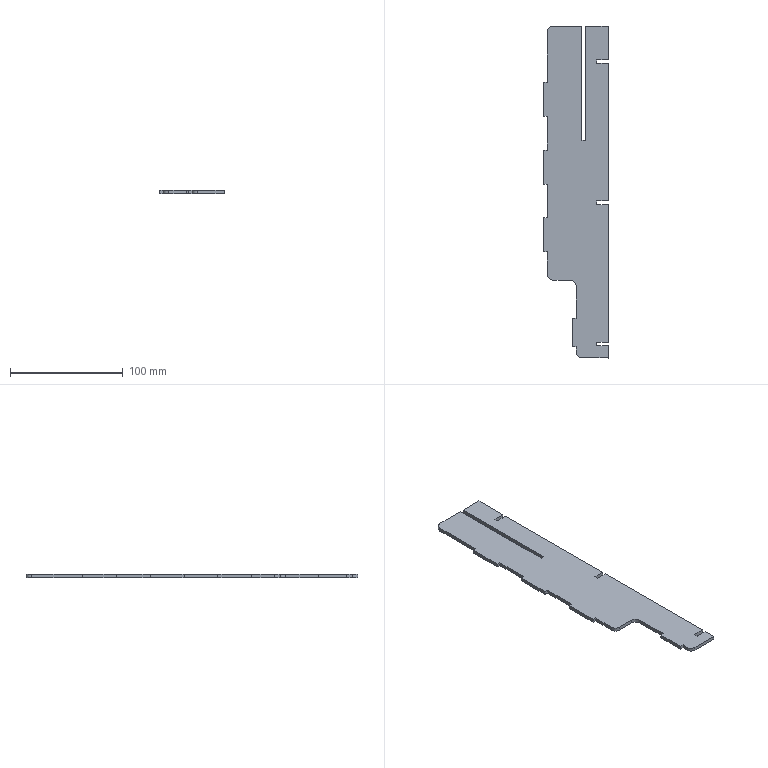Part | SolidWorks | features FlatPattern 1, SMBaseFlange 1, SheetMetal 1 | 1 solid | 44 faces | box 57 x 294.081 x 3.2 mm | volume 44908 mm3 | plane 40 | cylinder 4 | commonest cylinder face diameters 10 x4
STEP:
#1=CARTESIAN_POINT('',(-401.9,-209.357,0.));
#2=VERTEX_POINT('',#1);
#3=CARTESIAN_POINT('',(-378.4,-209.357,0.));
#4=VERTEX_POINT('',#3);
#5=CARTESIAN_POINT('',(-401.9,-209.357,0.));
#6=DIRECTION('',(1.,-0.00000003,0.));
#7=VECTOR('',#6,1000.);
#8=LINE('',#5,#7);
#9=EDGE_CURVE('',#2,#4,#8,.T.);
#10=ORIENTED_EDGE('',*,*,#9,.F.);
#11=CARTESIAN_POINT('',(-401.9,-209.357,-3.2));
#12=VERTEX_POINT('',#11);
#13=CARTESIAN_POINT('',(-401.9,-209.357,-3.2));
#14=DIRECTION('',(0.,0.,1.));
#15=VECTOR('',#14,1000.);
#16=LINE('',#13,#15);
#17=EDGE_CURVE('',#12,#2,#16,.T.);
#18=ORIENTED_EDGE('',*,*,#17,.F.);
#19=CARTESIAN_POINT('',(-378.4,-209.357,-3.2));
#20=VERTEX_POINT('',#19);
#21=CARTESIAN_POINT('',(-401.9,-209.357,-3.2));
#22=DIRECTION('',(1.,-0.00000003,0.));
#23=VECTOR('',#22,1000.);
#24=LINE('',#21,#23);
#25=EDGE_CURVE('',#12,#20,#24,.T.);
#26=ORIENTED_EDGE('',*,*,#25,.T.);
#27=CARTESIAN_POINT('',(-378.4,-209.357,-3.2));
#28=DIRECTION('',(0.,0.,1.));
#29=VECTOR('',#28,1000.);
#30=LINE('',#27,#29);
#31=EDGE_CURVE('',#20,#4,#30,.T.);
#32=ORIENTED_EDGE('',*,*,#31,.T.);
#33=EDGE_LOOP('',(#10,#18,#26,#32));
#34=FACE_OUTER_BOUND('',#33,.T.);
#35=CARTESIAN_POINT('',(-401.9,-209.357,-3.2));
#36=DIRECTION('',(-0.00000003,-1.,0.));
#37=DIRECTION('',(1.,-0.00000003,0.));
#38=AXIS2_PLACEMENT_3D('',#35,#36,#37);
#39=PLANE('',#38);
#40=ADVANCED_FACE('',(#34),#39,.T.);
#41=CARTESIAN_POINT('',(-406.9,-204.357,0.));
#42=VERTEX_POINT('',#41);
#43=CARTESIAN_POINT('',(-401.9,-204.357,0.));
#44=DIRECTION('',(0.,0.,1.));
#45=DIRECTION('',(-1.,0.,0.));
#46=AXIS2_PLACEMENT_3D('',#43,#44,#45);
#47=CIRCLE('',#46,5.);
#48=EDGE_CURVE('',#42,#2,#47,.T.);
#49=ORIENTED_EDGE('',*,*,#48,.F.);
#50=CARTESIAN_POINT('',(-406.9,-204.357,-3.2));
#51=VERTEX_POINT('',#50);
#52=CARTESIAN_POINT('',(-406.9,-204.357,-3.2));
#53=DIRECTION('',(0.,0.,1.));
#54=VECTOR('',#53,1000.);
#55=LINE('',#52,#54);
#56=EDGE_CURVE('',#51,#42,#55,.T.);
#57=ORIENTED_EDGE('',*,*,#56,.F.);
#58=CARTESIAN_POINT('',(-401.9,-204.357,-3.2));
#59=DIRECTION('',(0.,0.,1.));
#60=DIRECTION('',(-1.,0.,0.));
#61=AXIS2_PLACEMENT_3D('',#58,#59,#60);
#62=CIRCLE('',#61,5.);
#63=EDGE_CURVE('',#51,#12,#62,.T.);
#64=ORIENTED_EDGE('',*,*,#63,.T.);
#65=ORIENTED_EDGE('',*,*,#17,.T.);
#66=EDGE_LOOP('',(#49,#57,#64,#65));
#67=FACE_OUTER_BOUND('',#66,.T.);
#68=CARTESIAN_POINT('',(-401.9,-204.357,-3.2));
#69=DIRECTION('',(0.,0.,1.));
#70=DIRECTION('',(1.,0.,0.));
#71=AXIS2_PLACEMENT_3D('',#68,#69,#70);
#72=CYLINDRICAL_SURFACE('',#71,5.);
#73=ADVANCED_FACE('',(#67),#72,.T.);
#74=CARTESIAN_POINT('',(-406.9,-199.357,0.));
#75=VERTEX_POINT('',#74);
#76=CARTESIAN_POINT('',(-406.9,-199.357,0.));
#77=DIRECTION('',(0.,-1.,0.));
#78=VECTOR('',#77,1000.);
#79=LINE('',#76,#78);
#80=EDGE_CURVE('',#75,#42,#79,.T.);
#81=ORIENTED_EDGE('',*,*,#80,.F.);
#82=CARTESIAN_POINT('',(-406.9,-199.357,-3.2));
#83=VERTEX_POINT('',#82);
#84=CARTESIAN_POINT('',(-406.9,-199.357,-3.2));
#85=DIRECTION('',(0.,0.,1.));
#86=VECTOR('',#85,1000.);
#87=LINE('',#84,#86);
#88=EDGE_CURVE('',#83,#75,#87,.T.);
#89=ORIENTED_EDGE('',*,*,#88,.F.);
#90=CARTESIAN_POINT('',(-406.9,-199.357,-3.2));
#91=DIRECTION('',(0.,-1.,0.));
#92=VECTOR('',#91,1000.);
#93=LINE('',#90,#92);
#94=EDGE_CURVE('',#83,#51,#93,.T.);
#95=ORIENTED_EDGE('',*,*,#94,.T.);
#96=ORIENTED_EDGE('',*,*,#56,.T.);
#97=EDGE_LOOP('',(#81,#89,#95,#96));
#98=FACE_OUTER_BOUND('',#97,.T.);
#99=CARTESIAN_POINT('',(-406.9,-199.357,-3.2));
#100=DIRECTION('',(-1.,0.,0.));
#101=DIRECTION('',(0.,0.,1.));
#102=AXIS2_PLACEMENT_3D('',#99,#100,#101);
#103=PLANE('',#102);
#104=ADVANCED_FACE('',(#98),#103,.T.);
#105=CARTESIAN_POINT('',(-409.9,-199.357,0.));
#106=VERTEX_POINT('',#105);
#107=CARTESIAN_POINT('',(-409.9,-199.357,0.));
#108=DIRECTION('',(1.,0.,0.));
#109=VECTOR('',#108,1000.);
#110=LINE('',#107,#109);
#111=EDGE_CURVE('',#106,#75,#110,.T.);
#112=ORIENTED_EDGE('',*,*,#111,.F.);
#113=CARTESIAN_POINT('',(-409.9,-199.357,-3.2));
#114=VERTEX_POINT('',#113);
#115=CARTESIAN_POINT('',(-409.9,-199.357,-3.2));
#116=DIRECTION('',(0.,0.,1.));
#117=VECTOR('',#116,1000.);
#118=LINE('',#115,#117);
#119=EDGE_CURVE('',#114,#106,#118,.T.);
#120=ORIENTED_EDGE('',*,*,#119,.F.);
#121=CARTESIAN_POINT('',(-409.9,-199.357,-3.2));
#122=DIRECTION('',(1.,0.,0.));
#123=VECTOR('',#122,1000.);
#124=LINE('',#121,#123);
#125=EDGE_CURVE('',#114,#83,#124,.T.);
#126=ORIENTED_EDGE('',*,*,#125,.T.);
#127=ORIENTED_EDGE('',*,*,#88,.T.);
#128=EDGE_LOOP('',(#112,#120,#126,#127));
#129=FACE_OUTER_BOUND('',#128,.T.);
#130=CARTESIAN_POINT('',(-409.9,-199.357,-3.2));
#131=DIRECTION('',(0.,-1.,0.));
#132=DIRECTION('',(1.,0.,0.));
#133=AXIS2_PLACEMENT_3D('',#130,#131,#132);
#134=PLANE('',#133);
#135=ADVANCED_FACE('',(#129),#134,.T.);
#136=CARTESIAN_POINT('',(-409.9,-174.357,0.));
#137=VERTEX_POINT('',#136);
#138=CARTESIAN_POINT('',(-409.9,-174.357,0.));
#139=DIRECTION('',(0.,-1.,0.));
#140=VECTOR('',#139,1000.);
#141=LINE('',#138,#140);
#142=EDGE_CURVE('',#137,#106,#141,.T.);
#143=ORIENTED_EDGE('',*,*,#142,.F.);
#144=CARTESIAN_POINT('',(-409.9,-174.357,-3.2));
#145=VERTEX_POINT('',#144);
#146=CARTESIAN_POINT('',(-409.9,-174.357,-3.2));
#147=DIRECTION('',(0.,0.,1.));
#148=VECTOR('',#147,1000.);
#149=LINE('',#146,#148);
#150=EDGE_CURVE('',#145,#137,#149,.T.);
#151=ORIENTED_EDGE('',*,*,#150,.F.);
#152=CARTESIAN_POINT('',(-409.9,-174.357,-3.2));
#153=DIRECTION('',(0.,-1.,0.));
#154=VECTOR('',#153,1000.);
#155=LINE('',#152,#154);
#156=EDGE_CURVE('',#145,#114,#155,.T.);
#157=ORIENTED_EDGE('',*,*,#156,.T.);
#158=ORIENTED_EDGE('',*,*,#119,.T.);
#159=EDGE_LOOP('',(#143,#151,#157,#158));
#160=FACE_OUTER_BOUND('',#159,.T.);
#161=CARTESIAN_POINT('',(-409.9,-174.357,-3.2));
#162=DIRECTION('',(-1.,0.,0.));
#163=DIRECTION('',(0.,-1.,0.));
#164=AXIS2_PLACEMENT_3D('',#161,#162,#163);
#165=PLANE('',#164);
#166=ADVANCED_FACE('',(#160),#165,.T.);
#167=CARTESIAN_POINT('',(-406.9,-174.357,0.));
#168=VERTEX_POINT('',#167);
#169=CARTESIAN_POINT('',(-406.9,-174.357,0.));
#170=DIRECTION('',(-1.,0.,0.));
#171=VECTOR('',#170,1000.);
#172=LINE('',#169,#171);
#173=EDGE_CURVE('',#168,#137,#172,.T.);
#174=ORIENTED_EDGE('',*,*,#173,.F.);
#175=CARTESIAN_POINT('',(-406.9,-174.357,-3.2));
#176=VERTEX_POINT('',#175);
#177=CARTESIAN_POINT('',(-406.9,-174.357,-3.2));
#178=DIRECTION('',(0.,0.,1.));
#179=VECTOR('',#178,1000.);
#180=LINE('',#177,#179);
#181=EDGE_CURVE('',#176,#168,#180,.T.);
#182=ORIENTED_EDGE('',*,*,#181,.F.);
#183=CARTESIAN_POINT('',(-406.9,-174.357,-3.2));
#184=DIRECTION('',(-1.,0.,0.));
#185=VECTOR('',#184,1000.);
#186=LINE('',#183,#185);
#187=EDGE_CURVE('',#176,#145,#186,.T.);
#188=ORIENTED_EDGE('',*,*,#187,.T.);
#189=ORIENTED_EDGE('',*,*,#150,.T.);
#190=EDGE_LOOP('',(#174,#182,#188,#189));
#191=FACE_OUTER_BOUND('',#190,.T.);
#192=CARTESIAN_POINT('',(-406.9,-174.357,-3.2));
#193=DIRECTION('',(0.,1.,0.));
#194=DIRECTION('',(0.,0.,1.));
#195=AXIS2_PLACEMENT_3D('',#192,#193,#194);
#196=PLANE('',#195);
#197=ADVANCED_FACE('',(#191),#196,.T.);
#198=CARTESIAN_POINT('',(-406.9,-145.276,0.));
#199=VERTEX_POINT('',#198);
#200=CARTESIAN_POINT('',(-406.9,-145.276,0.));
#201=DIRECTION('',(0.000000012,-1.,0.));
#202=VECTOR('',#201,1000.);
#203=LINE('',#200,#202);
#204=EDGE_CURVE('',#199,#168,#203,.T.);
#205=ORIENTED_EDGE('',*,*,#204,.F.);
#206=CARTESIAN_POINT('',(-406.9,-145.276,-3.2));
#207=VERTEX_POINT('',#206);
#208=CARTESIAN_POINT('',(-406.9,-145.276,-3.2));
#209=DIRECTION('',(0.,0.,1.));
#210=VECTOR('',#209,1000.);
#211=LINE('',#208,#210);
#212=EDGE_CURVE('',#207,#199,#211,.T.);
#213=ORIENTED_EDGE('',*,*,#212,.F.);
#214=CARTESIAN_POINT('',(-406.9,-145.276,-3.2));
#215=DIRECTION('',(0.000000012,-1.,0.));
#216=VECTOR('',#215,1000.);
#217=LINE('',#214,#216);
#218=EDGE_CURVE('',#207,#176,#217,.T.);
#219=ORIENTED_EDGE('',*,*,#218,.T.);
#220=ORIENTED_EDGE('',*,*,#181,.T.);
#221=EDGE_LOOP('',(#205,#213,#219,#220));
#222=FACE_OUTER_BOUND('',#221,.T.);
#223=CARTESIAN_POINT('',(-406.9,-145.276,-3.2));
#224=DIRECTION('',(-1.,-0.000000012,0.));
#225=DIRECTION('',(0.000000012,-1.,0.));
#226=AXIS2_PLACEMENT_3D('',#223,#224,#225);
#227=PLANE('',#226);
#228=ADVANCED_FACE('',(#222),#227,.T.);
#229=CARTESIAN_POINT('',(-411.9,-140.276,0.));
#230=VERTEX_POINT('',#229);
#231=CARTESIAN_POINT('',(-411.9,-145.276,0.));
#232=DIRECTION('',(0.,0.,-1.));
#233=DIRECTION('',(-1.,0.,0.));
#234=AXIS2_PLACEMENT_3D('',#231,#232,#233);
#235=CIRCLE('',#234,5.);
#236=EDGE_CURVE('',#230,#199,#235,.T.);
#237=ORIENTED_EDGE('',*,*,#236,.F.);
#238=CARTESIAN_POINT('',(-411.9,-140.276,-3.2));
#239=VERTEX_POINT('',#238);
#240=CARTESIAN_POINT('',(-411.9,-140.276,-3.2));
#241=DIRECTION('',(0.,0.,1.));
#242=VECTOR('',#241,1000.);
#243=LINE('',#240,#242);
#244=EDGE_CURVE('',#239,#230,#243,.T.);
#245=ORIENTED_EDGE('',*,*,#244,.F.);
#246=CARTESIAN_POINT('',(-411.9,-145.276,-3.2));
#247=DIRECTION('',(0.,0.,-1.));
#248=DIRECTION('',(-1.,0.,0.));
#249=AXIS2_PLACEMENT_3D('',#246,#247,#248);
#250=CIRCLE('',#249,5.);
#251=EDGE_CURVE('',#239,#207,#250,.T.);
#252=ORIENTED_EDGE('',*,*,#251,.T.);
#253=ORIENTED_EDGE('',*,*,#212,.T.);
#254=EDGE_LOOP('',(#237,#245,#252,#253));
#255=FACE_OUTER_BOUND('',#254,.T.);
#256=CARTESIAN_POINT('',(-411.9,-145.276,-3.2));
#257=DIRECTION('',(0.,0.,1.));
#258=DIRECTION('',(1.,0.,0.));
#259=AXIS2_PLACEMENT_3D('',#256,#257,#258);
#260=CYLINDRICAL_SURFACE('',#259,5.);
#261=ADVANCED_FACE('',(#255),#260,.F.);
#262=CARTESIAN_POINT('',(-427.4,-140.276,0.));
#263=VERTEX_POINT('',#262);
#264=CARTESIAN_POINT('',(-427.4,-140.276,0.));
#265=DIRECTION('',(1.,0.,0.));
#266=VECTOR('',#265,1000.);
#267=LINE('',#264,#266);
#268=EDGE_CURVE('',#263,#230,#267,.T.);
#269=ORIENTED_EDGE('',*,*,#268,.F.);
#270=CARTESIAN_POINT('',(-427.4,-140.276,-3.2));
#271=VERTEX_POINT('',#270);
#272=CARTESIAN_POINT('',(-427.4,-140.276,-3.2));
#273=DIRECTION('',(0.,0.,1.));
#274=VECTOR('',#273,1000.);
#275=LINE('',#272,#274);
#276=EDGE_CURVE('',#271,#263,#275,.T.);
#277=ORIENTED_EDGE('',*,*,#276,.F.);
#278=CARTESIAN_POINT('',(-427.4,-140.276,-3.2));
#279=DIRECTION('',(1.,0.,0.));
#280=VECTOR('',#279,1000.);
#281=LINE('',#278,#280);
#282=EDGE_CURVE('',#271,#239,#281,.T.);
#283=ORIENTED_EDGE('',*,*,#282,.T.);
#284=ORIENTED_EDGE('',*,*,#244,.T.);
#285=EDGE_LOOP('',(#269,#277,#283,#284));
#286=FACE_OUTER_BOUND('',#285,.T.);
#287=CARTESIAN_POINT('',(-427.4,-140.276,-3.2));
#288=DIRECTION('',(0.,-1.,0.));
#289=DIRECTION('',(0.,0.,-1.));
#290=AXIS2_PLACEMENT_3D('',#287,#288,#289);
#291=PLANE('',#290);
#292=ADVANCED_FACE('',(#286),#291,.T.);
#293=CARTESIAN_POINT('',(-432.4,-135.276,0.));
#294=VERTEX_POINT('',#293);
#295=CARTESIAN_POINT('',(-427.4,-135.276,0.));
#296=DIRECTION('',(0.,0.,1.));
#297=DIRECTION('',(-1.,0.,0.));
#298=AXIS2_PLACEMENT_3D('',#295,#296,#297);
#299=CIRCLE('',#298,5.);
#300=EDGE_CURVE('',#294,#263,#299,.T.);
#301=ORIENTED_EDGE('',*,*,#300,.F.);
#302=CARTESIAN_POINT('',(-432.4,-135.276,-3.2));
#303=VERTEX_POINT('',#302);
#304=CARTESIAN_POINT('',(-432.4,-135.276,-3.2));
#305=DIRECTION('',(0.,0.,1.));
#306=VECTOR('',#305,1000.);
#307=LINE('',#304,#306);
#308=EDGE_CURVE('',#303,#294,#307,.T.);
#309=ORIENTED_EDGE('',*,*,#308,.F.);
#310=CARTESIAN_POINT('',(-427.4,-135.276,-3.2));
#311=DIRECTION('',(0.,0.,1.));
#312=DIRECTION('',(-1.,0.,0.));
#313=AXIS2_PLACEMENT_3D('',#310,#311,#312);
#314=CIRCLE('',#313,5.);
#315=EDGE_CURVE('',#303,#271,#314,.T.);
#316=ORIENTED_EDGE('',*,*,#315,.T.);
#317=ORIENTED_EDGE('',*,*,#276,.T.);
#318=EDGE_LOOP('',(#301,#309,#316,#317));
#319=FACE_OUTER_BOUND('',#318,.T.);
#320=CARTESIAN_POINT('',(-427.4,-135.276,-3.2));
#321=DIRECTION('',(0.,0.,1.));
#322=DIRECTION('',(1.,0.,0.));
#323=AXIS2_PLACEMENT_3D('',#320,#321,#322);
#324=CYLINDRICAL_SURFACE('',#323,5.);
#325=ADVANCED_FACE('',(#319),#324,.T.);
#326=CARTESIAN_POINT('',(-432.4,-115.276,0.));
#327=VERTEX_POINT('',#326);
#328=CARTESIAN_POINT('',(-432.4,-135.276,0.));
#329=DIRECTION('',(0.,-1.,0.));
#330=VECTOR('',#329,1000.);
#331=LINE('',#328,#330);
#332=EDGE_CURVE('',#327,#294,#331,.T.);
#333=ORIENTED_EDGE('',*,*,#332,.F.);
#334=CARTESIAN_POINT('',(-432.4,-115.276,-3.2));
#335=VERTEX_POINT('',#334);
#336=CARTESIAN_POINT('',(-432.4,-115.276,-3.2));
#337=DIRECTION('',(0.,0.,1.));
#338=VECTOR('',#337,1000.);
#339=LINE('',#336,#338);
#340=EDGE_CURVE('',#335,#327,#339,.T.);
#341=ORIENTED_EDGE('',*,*,#340,.F.);
#342=CARTESIAN_POINT('',(-432.4,-135.276,-3.2));
#343=DIRECTION('',(0.,-1.,0.));
#344=VECTOR('',#343,1000.);
#345=LINE('',#342,#344);
#346=EDGE_CURVE('',#335,#303,#345,.T.);
#347=ORIENTED_EDGE('',*,*,#346,.T.);
#348=ORIENTED_EDGE('',*,*,#308,.T.);
#349=EDGE_LOOP('',(#333,#341,#347,#348));
#350=FACE_OUTER_BOUND('',#349,.T.);
#351=CARTESIAN_POINT('',(-432.4,-135.276,-3.2));
#352=DIRECTION('',(-1.,0.,0.));
#353=DIRECTION('',(0.,0.,1.));
#354=AXIS2_PLACEMENT_3D('',#351,#352,#353);
#355=PLANE('',#354);
#356=ADVANCED_FACE('',(#350),#355,.T.);
#357=CARTESIAN_POINT('',(-435.4,-115.276,0.));
#358=VERTEX_POINT('',#357);
#359=CARTESIAN_POINT('',(-435.4,-115.276,0.));
#360=DIRECTION('',(1.,0.,0.));
#361=VECTOR('',#360,1000.);
#362=LINE('',#359,#361);
#363=EDGE_CURVE('',#358,#327,#362,.T.);
#364=ORIENTED_EDGE('',*,*,#363,.F.);
#365=CARTESIAN_POINT('',(-435.4,-115.276,-3.2));
#366=VERTEX_POINT('',#365);
#367=CARTESIAN_POINT('',(-435.4,-115.276,-3.2));
#368=DIRECTION('',(0.,0.,1.));
#369=VECTOR('',#368,1000.);
#370=LINE('',#367,#369);
#371=EDGE_CURVE('',#366,#358,#370,.T.);
#372=ORIENTED_EDGE('',*,*,#371,.F.);
#373=CARTESIAN_POINT('',(-435.4,-115.276,-3.2));
#374=DIRECTION('',(1.,0.,0.));
#375=VECTOR('',#374,1000.);
#376=LINE('',#373,#375);
#377=EDGE_CURVE('',#366,#335,#376,.T.);
#378=ORIENTED_EDGE('',*,*,#377,.T.);
#379=ORIENTED_EDGE('',*,*,#340,.T.);
#380=EDGE_LOOP('',(#364,#372,#378,#379));
#381=FACE_OUTER_BOUND('',#380,.T.);
#382=CARTESIAN_POINT('',(-435.4,-115.276,-3.2));
#383=DIRECTION('',(0.,-1.,0.));
#384=DIRECTION('',(0.,0.,-1.));
#385=AXIS2_PLACEMENT_3D('',#382,#383,#384);
#386=PLANE('',#385);
#387=ADVANCED_FACE('',(#381),#386,.T.);
#388=CARTESIAN_POINT('',(-435.4,-85.276,0.));
#389=VERTEX_POINT('',#388);
#390=CARTESIAN_POINT('',(-435.4,-85.276,0.));
#391=DIRECTION('',(0.,-1.,0.));
#392=VECTOR('',#391,1000.);
#393=LINE('',#390,#392);
#394=EDGE_CURVE('',#389,#358,#393,.T.);
#395=ORIENTED_EDGE('',*,*,#394,.F.);
#396=CARTESIAN_POINT('',(-435.4,-85.276,-3.2));
#397=VERTEX_POINT('',#396);
#398=CARTESIAN_POINT('',(-435.4,-85.276,-3.2));
#399=DIRECTION('',(0.,0.,1.));
#400=VECTOR('',#399,1000.);
#401=LINE('',#398,#400);
#402=EDGE_CURVE('',#397,#389,#401,.T.);
#403=ORIENTED_EDGE('',*,*,#402,.F.);
#404=CARTESIAN_POINT('',(-435.4,-85.276,-3.2));
#405=DIRECTION('',(0.,-1.,0.));
#406=VECTOR('',#405,1000.);
#407=LINE('',#404,#406);
#408=EDGE_CURVE('',#397,#366,#407,.T.);
#409=ORIENTED_EDGE('',*,*,#408,.T.);
#410=ORIENTED_EDGE('',*,*,#371,.T.);
#411=EDGE_LOOP('',(#395,#403,#409,#410));
#412=FACE_OUTER_BOUND('',#411,.T.);
#413=CARTESIAN_POINT('',(-435.4,-85.276,-3.2));
#414=DIRECTION('',(-1.,0.,0.));
#415=DIRECTION('',(0.,0.,1.));
#416=AXIS2_PLACEMENT_3D('',#413,#414,#415);
#417=PLANE('',#416);
#418=ADVANCED_FACE('',(#412),#417,.T.);
#419=CARTESIAN_POINT('',(-432.4,-85.276,0.));
#420=VERTEX_POINT('',#419);
#421=CARTESIAN_POINT('',(-432.4,-85.276,0.));
#422=DIRECTION('',(-1.,0.,0.));
#423=VECTOR('',#422,1000.);
#424=LINE('',#421,#423);
#425=EDGE_CURVE('',#420,#389,#424,.T.);
#426=ORIENTED_EDGE('',*,*,#425,.F.);
#427=CARTESIAN_POINT('',(-432.4,-85.276,-3.2));
#428=VERTEX_POINT('',#427);
#429=CARTESIAN_POINT('',(-432.4,-85.276,-3.2));
#430=DIRECTION('',(0.,0.,1.));
#431=VECTOR('',#430,1000.);
#432=LINE('',#429,#431);
#433=EDGE_CURVE('',#428,#420,#432,.T.);
#434=ORIENTED_EDGE('',*,*,#433,.F.);
#435=CARTESIAN_POINT('',(-432.4,-85.276,-3.2));
#436=DIRECTION('',(-1.,0.,0.));
#437=VECTOR('',#436,1000.);
#438=LINE('',#435,#437);
#439=EDGE_CURVE('',#428,#397,#438,.T.);
#440=ORIENTED_EDGE('',*,*,#439,.T.);
#441=ORIENTED_EDGE('',*,*,#402,.T.);
#442=EDGE_LOOP('',(#426,#434,#440,#441));
#443=FACE_OUTER_BOUND('',#442,.T.);
#444=CARTESIAN_POINT('',(-432.4,-85.276,-3.2));
#445=DIRECTION('',(0.,1.,0.));
#446=DIRECTION('',(0.,0.,1.));
#447=AXIS2_PLACEMENT_3D('',#444,#445,#446);
#448=PLANE('',#447);
#449=ADVANCED_FACE('',(#443),#448,.T.);
#450=CARTESIAN_POINT('',(-432.4,-55.276,0.));
#451=VERTEX_POINT('',#450);
#452=CARTESIAN_POINT('',(-432.4,-85.276,0.));
#453=DIRECTION('',(0.,-1.,0.));
#454=VECTOR('',#453,1000.);
#455=LINE('',#452,#454);
#456=EDGE_CURVE('',#451,#420,#455,.T.);
#457=ORIENTED_EDGE('',*,*,#456,.F.);
#458=CARTESIAN_POINT('',(-432.4,-55.276,-3.2));
#459=VERTEX_POINT('',#458);
#460=CARTESIAN_POINT('',(-432.4,-55.276,-3.2));
#461=DIRECTION('',(0.,0.,1.));
#462=VECTOR('',#461,1000.);
#463=LINE('',#460,#462);
#464=EDGE_CURVE('',#459,#451,#463,.T.);
#465=ORIENTED_EDGE('',*,*,#464,.F.);
#466=CARTESIAN_POINT('',(-432.4,-85.276,-3.2));
#467=DIRECTION('',(0.,-1.,0.));
#468=VECTOR('',#467,1000.);
#469=LINE('',#466,#468);
#470=EDGE_CURVE('',#459,#428,#469,.T.);
#471=ORIENTED_EDGE('',*,*,#470,.T.);
#472=ORIENTED_EDGE('',*,*,#433,.T.);
#473=EDGE_LOOP('',(#457,#465,#471,#472));
#474=FACE_OUTER_BOUND('',#473,.T.);
#475=CARTESIAN_POINT('',(-432.4,-85.276,-3.2));
#476=DIRECTION('',(-1.,0.,0.));
#477=DIRECTION('',(0.,0.,1.));
#478=AXIS2_PLACEMENT_3D('',#475,#476,#477);
#479=PLANE('',#478);
#480=ADVANCED_FACE('',(#474),#479,.T.);
#481=CARTESIAN_POINT('',(-435.4,-55.276,0.));
#482=VERTEX_POINT('',#481);
#483=CARTESIAN_POINT('',(-435.4,-55.276,0.));
#484=DIRECTION('',(1.,0.,0.));
#485=VECTOR('',#484,1000.);
#486=LINE('',#483,#485);
#487=EDGE_CURVE('',#482,#451,#486,.T.);
#488=ORIENTED_EDGE('',*,*,#487,.F.);
#489=CARTESIAN_POINT('',(-435.4,-55.276,-3.2));
#490=VERTEX_POINT('',#489);
#491=CARTESIAN_POINT('',(-435.4,-55.276,-3.2));
#492=DIRECTION('',(0.,0.,1.));
#493=VECTOR('',#492,1000.);
#494=LINE('',#491,#493);
#495=EDGE_CURVE('',#490,#482,#494,.T.);
#496=ORIENTED_EDGE('',*,*,#495,.F.);
#497=CARTESIAN_POINT('',(-435.4,-55.276,-3.2));
#498=DIRECTION('',(1.,0.,0.));
#499=VECTOR('',#498,1000.);
#500=LINE('',#497,#499);
#501=EDGE_CURVE('',#490,#459,#500,.T.);
#502=ORIENTED_EDGE('',*,*,#501,.T.);
#503=ORIENTED_EDGE('',*,*,#464,.T.);
#504=EDGE_LOOP('',(#488,#496,#502,#503));
#505=FACE_OUTER_BOUND('',#504,.T.);
#506=CARTESIAN_POINT('',(-435.4,-55.276,-3.2));
#507=DIRECTION('',(0.,-1.,0.));
#508=DIRECTION('',(0.,0.,-1.));
#509=AXIS2_PLACEMENT_3D('',#506,#507,#508);
#510=PLANE('',#509);
#511=ADVANCED_FACE('',(#505),#510,.T.);
#512=CARTESIAN_POINT('',(-435.4,-25.276,0.));
#513=VERTEX_POINT('',#512);
#514=CARTESIAN_POINT('',(-435.4,-25.276,0.));
#515=DIRECTION('',(0.,-1.,0.));
#516=VECTOR('',#515,1000.);
#517=LINE('',#514,#516);
#518=EDGE_CURVE('',#513,#482,#517,.T.);
#519=ORIENTED_EDGE('',*,*,#518,.F.);
#520=CARTESIAN_POINT('',(-435.4,-25.276,-3.2));
#521=VERTEX_POINT('',#520);
#522=CARTESIAN_POINT('',(-435.4,-25.276,-3.2));
#523=DIRECTION('',(0.,0.,1.));
#524=VECTOR('',#523,1000.);
#525=LINE('',#522,#524);
#526=EDGE_CURVE('',#521,#513,#525,.T.);
#527=ORIENTED_EDGE('',*,*,#526,.F.);
#528=CARTESIAN_POINT('',(-435.4,-25.276,-3.2));
#529=DIRECTION('',(0.,-1.,0.));
#530=VECTOR('',#529,1000.);
#531=LINE('',#528,#530);
#532=EDGE_CURVE('',#521,#490,#531,.T.);
#533=ORIENTED_EDGE('',*,*,#532,.T.);
#534=ORIENTED_EDGE('',*,*,#495,.T.);
#535=EDGE_LOOP('',(#519,#527,#533,#534));
#536=FACE_OUTER_BOUND('',#535,.T.);
#537=CARTESIAN_POINT('',(-435.4,-25.276,-3.2));
#538=DIRECTION('',(-1.,0.,0.));
#539=DIRECTION('',(0.,0.,1.));
#540=AXIS2_PLACEMENT_3D('',#537,#538,#539);
#541=PLANE('',#540);
#542=ADVANCED_FACE('',(#536),#541,.T.);
#543=CARTESIAN_POINT('',(-432.4,-25.276,0.));
#544=VERTEX_POINT('',#543);
#545=CARTESIAN_POINT('',(-432.4,-25.276,0.));
#546=DIRECTION('',(-1.,0.,0.));
#547=VECTOR('',#546,1000.);
#548=LINE('',#545,#547);
#549=EDGE_CURVE('',#544,#513,#548,.T.);
#550=ORIENTED_EDGE('',*,*,#549,.F.);
#551=CARTESIAN_POINT('',(-432.4,-25.276,-3.2));
#552=VERTEX_POINT('',#551);
#553=CARTESIAN_POINT('',(-432.4,-25.276,-3.2));
#554=DIRECTION('',(0.,0.,1.));
#555=VECTOR('',#554,1000.);
#556=LINE('',#553,#555);
#557=EDGE_CURVE('',#552,#544,#556,.T.);
#558=ORIENTED_EDGE('',*,*,#557,.F.);
#559=CARTESIAN_POINT('',(-432.4,-25.276,-3.2));
#560=DIRECTION('',(-1.,0.,0.));
#561=VECTOR('',#560,1000.);
#562=LINE('',#559,#561);
#563=EDGE_CURVE('',#552,#521,#562,.T.);
#564=ORIENTED_EDGE('',*,*,#563,.T.);
#565=ORIENTED_EDGE('',*,*,#526,.T.);
#566=EDGE_LOOP('',(#550,#558,#564,#565));
#567=FACE_OUTER_BOUND('',#566,.T.);
#568=CARTESIAN_POINT('',(-432.4,-25.276,-3.2));
#569=DIRECTION('',(0.,1.,0.));
#570=DIRECTION('',(0.,0.,1.));
#571=AXIS2_PLACEMENT_3D('',#568,#569,#570);
#572=PLANE('',#571);
#573=ADVANCED_FACE('',(#567),#572,.T.);
#574=CARTESIAN_POINT('',(-432.4,4.724,0.));
#575=VERTEX_POINT('',#574);
#576=CARTESIAN_POINT('',(-432.4,-25.276,0.));
#577=DIRECTION('',(0.,-1.,0.));
#578=VECTOR('',#577,1000.);
#579=LINE('',#576,#578);
#580=EDGE_CURVE('',#575,#544,#579,.T.);
#581=ORIENTED_EDGE('',*,*,#580,.F.);
#582=CARTESIAN_POINT('',(-432.4,4.724,-3.2));
#583=VERTEX_POINT('',#582);
#584=CARTESIAN_POINT('',(-432.4,4.724,-3.2));
#585=DIRECTION('',(0.,0.,1.));
#586=VECTOR('',#585,1000.);
#587=LINE('',#584,#586);
#588=EDGE_CURVE('',#583,#575,#587,.T.);
#589=ORIENTED_EDGE('',*,*,#588,.F.);
#590=CARTESIAN_POINT('',(-432.4,-25.276,-3.2));
#591=DIRECTION('',(0.,-1.,0.));
#592=VECTOR('',#591,1000.);
#593=LINE('',#590,#592);
#594=EDGE_CURVE('',#583,#552,#593,.T.);
#595=ORIENTED_EDGE('',*,*,#594,.T.);
#596=ORIENTED_EDGE('',*,*,#557,.T.);
#597=EDGE_LOOP('',(#581,#589,#595,#596));
#598=FACE_OUTER_BOUND('',#597,.T.);
#599=CARTESIAN_POINT('',(-432.4,-25.276,-3.2));
#600=DIRECTION('',(-1.,0.,0.));
#601=DIRECTION('',(0.,0.,1.));
#602=AXIS2_PLACEMENT_3D('',#599,#600,#601);
#603=PLANE('',#602);
#604=ADVANCED_FACE('',(#598),#603,.T.);
#605=CARTESIAN_POINT('',(-435.4,4.724,0.));
#606=VERTEX_POINT('',#605);
#607=CARTESIAN_POINT('',(-435.4,4.724,0.));
#608=DIRECTION('',(1.,0.,0.));
#609=VECTOR('',#608,1000.);
#610=LINE('',#607,#609);
#611=EDGE_CURVE('',#606,#575,#610,.T.);
#612=ORIENTED_EDGE('',*,*,#611,.F.);
#613=CARTESIAN_POINT('',(-435.4,4.724,-3.2));
#614=VERTEX_POINT('',#613);
#615=CARTESIAN_POINT('',(-435.4,4.724,-3.2));
#616=DIRECTION('',(0.,0.,1.));
#617=VECTOR('',#616,1000.);
#618=LINE('',#615,#617);
#619=EDGE_CURVE('',#614,#606,#618,.T.);
#620=ORIENTED_EDGE('',*,*,#619,.F.);
#621=CARTESIAN_POINT('',(-435.4,4.724,-3.2));
#622=DIRECTION('',(1.,0.,0.));
#623=VECTOR('',#622,1000.);
#624=LINE('',#621,#623);
#625=EDGE_CURVE('',#614,#583,#624,.T.);
#626=ORIENTED_EDGE('',*,*,#625,.T.);
#627=ORIENTED_EDGE('',*,*,#588,.T.);
#628=EDGE_LOOP('',(#612,#620,#626,#627));
#629=FACE_OUTER_BOUND('',#628,.T.);
#630=CARTESIAN_POINT('',(-435.4,4.724,-3.2));
#631=DIRECTION('',(0.,-1.,0.));
#632=DIRECTION('',(0.,0.,-1.));
#633=AXIS2_PLACEMENT_3D('',#630,#631,#632);
#634=PLANE('',#633);
#635=ADVANCED_FACE('',(#629),#634,.T.);
#636=CARTESIAN_POINT('',(-435.4,34.724,0.));
#637=VERTEX_POINT('',#636);
#638=CARTESIAN_POINT('',(-435.4,34.724,0.));
#639=DIRECTION('',(0.,-1.,0.));
#640=VECTOR('',#639,1000.);
#641=LINE('',#638,#640);
#642=EDGE_CURVE('',#637,#606,#641,.T.);
#643=ORIENTED_EDGE('',*,*,#642,.F.);
#644=CARTESIAN_POINT('',(-435.4,34.724,-3.2));
#645=VERTEX_POINT('',#644);
#646=CARTESIAN_POINT('',(-435.4,34.724,-3.2));
#647=DIRECTION('',(0.,0.,1.));
#648=VECTOR('',#647,1000.);
#649=LINE('',#646,#648);
#650=EDGE_CURVE('',#645,#637,#649,.T.);
#651=ORIENTED_EDGE('',*,*,#650,.F.);
#652=CARTESIAN_POINT('',(-435.4,34.724,-3.2));
#653=DIRECTION('',(0.,-1.,0.));
#654=VECTOR('',#653,1000.);
#655=LINE('',#652,#654);
#656=EDGE_CURVE('',#645,#614,#655,.T.);
#657=ORIENTED_EDGE('',*,*,#656,.T.);
#658=ORIENTED_EDGE('',*,*,#619,.T.);
#659=EDGE_LOOP('',(#643,#651,#657,#658));
#660=FACE_OUTER_BOUND('',#659,.T.);
#661=CARTESIAN_POINT('',(-435.4,34.724,-3.2));
#662=DIRECTION('',(-1.,0.,0.));
#663=DIRECTION('',(0.,0.,1.));
#664=AXIS2_PLACEMENT_3D('',#661,#662,#663);
#665=PLANE('',#664);
#666=ADVANCED_FACE('',(#660),#665,.T.);
#667=CARTESIAN_POINT('',(-432.4,34.724,0.));
#668=VERTEX_POINT('',#667);
#669=CARTESIAN_POINT('',(-432.4,34.724,0.));
#670=DIRECTION('',(-1.,0.,0.));
#671=VECTOR('',#670,1000.);
#672=LINE('',#669,#671);
#673=EDGE_CURVE('',#668,#637,#672,.T.);
#674=ORIENTED_EDGE('',*,*,#673,.F.);
#675=CARTESIAN_POINT('',(-432.4,34.724,-3.2));
#676=VERTEX_POINT('',#675);
#677=CARTESIAN_POINT('',(-432.4,34.724,-3.2));
#678=DIRECTION('',(0.,0.,1.));
#679=VECTOR('',#678,1000.);
#680=LINE('',#677,#679);
#681=EDGE_CURVE('',#676,#668,#680,.T.);
#682=ORIENTED_EDGE('',*,*,#681,.F.);
#683=CARTESIAN_POINT('',(-432.4,34.724,-3.2));
#684=DIRECTION('',(-1.,0.,0.));
#685=VECTOR('',#684,1000.);
#686=LINE('',#683,#685);
#687=EDGE_CURVE('',#676,#645,#686,.T.);
#688=ORIENTED_EDGE('',*,*,#687,.T.);
#689=ORIENTED_EDGE('',*,*,#650,.T.);
#690=EDGE_LOOP('',(#674,#682,#688,#689));
#691=FACE_OUTER_BOUND('',#690,.T.);
#692=CARTESIAN_POINT('',(-432.4,34.724,-3.2));
#693=DIRECTION('',(0.,1.,0.));
#694=DIRECTION('',(0.,0.,1.));
#695=AXIS2_PLACEMENT_3D('',#692,#693,#694);
#696=PLANE('',#695);
#697=ADVANCED_FACE('',(#691),#696,.T.);
#698=CARTESIAN_POINT('',(-432.4,79.724,0.));
#699=VERTEX_POINT('',#698);
#700=CARTESIAN_POINT('',(-432.4,34.724,0.));
#701=DIRECTION('',(0.,-1.,0.));
#702=VECTOR('',#701,1000.);
#703=LINE('',#700,#702);
#704=EDGE_CURVE('',#699,#668,#703,.T.);
#705=ORIENTED_EDGE('',*,*,#704,.F.);
#706=CARTESIAN_POINT('',(-432.4,79.724,-3.2));
#707=VERTEX_POINT('',#706);
#708=CARTESIAN_POINT('',(-432.4,79.724,-3.2));
#709=DIRECTION('',(0.,0.,1.));
#710=VECTOR('',#709,1000.);
#711=LINE('',#708,#710);
#712=EDGE_CURVE('',#707,#699,#711,.T.);
#713=ORIENTED_EDGE('',*,*,#712,.F.);
#714=CARTESIAN_POINT('',(-432.4,34.724,-3.2));
#715=DIRECTION('',(0.,-1.,0.));
#716=VECTOR('',#715,1000.);
#717=LINE('',#714,#716);
#718=EDGE_CURVE('',#707,#676,#717,.T.);
#719=ORIENTED_EDGE('',*,*,#718,.T.);
#720=ORIENTED_EDGE('',*,*,#681,.T.);
#721=EDGE_LOOP('',(#705,#713,#719,#720));
#722=FACE_OUTER_BOUND('',#721,.T.);
#723=CARTESIAN_POINT('',(-432.4,34.724,-3.2));
#724=DIRECTION('',(-1.,0.,0.));
#725=DIRECTION('',(0.,0.,1.));
#726=AXIS2_PLACEMENT_3D('',#723,#724,#725);
#727=PLANE('',#726);
#728=ADVANCED_FACE('',(#722),#727,.T.);
#729=CARTESIAN_POINT('',(-427.4,84.724,0.));
#730=VERTEX_POINT('',#729);
#731=CARTESIAN_POINT('',(-427.4,79.724,0.));
#732=DIRECTION('',(0.,0.,1.));
#733=DIRECTION('',(1.,0.,0.));
#734=AXIS2_PLACEMENT_3D('',#731,#732,#733);
#735=CIRCLE('',#734,5.);
#736=EDGE_CURVE('',#730,#699,#735,.T.);
#737=ORIENTED_EDGE('',*,*,#736,.F.);
#738=CARTESIAN_POINT('',(-427.4,84.724,-3.2));
#739=VERTEX_POINT('',#738);
#740=CARTESIAN_POINT('',(-427.4,84.724,-3.2));
#741=DIRECTION('',(0.,0.,1.));
#742=VECTOR('',#741,1000.);
#743=LINE('',#740,#742);
#744=EDGE_CURVE('',#739,#730,#743,.T.);
#745=ORIENTED_EDGE('',*,*,#744,.F.);
#746=CARTESIAN_POINT('',(-427.4,79.724,-3.2));
#747=DIRECTION('',(0.,0.,1.));
#748=DIRECTION('',(1.,0.,0.));
#749=AXIS2_PLACEMENT_3D('',#746,#747,#748);
#750=CIRCLE('',#749,5.);
#751=EDGE_CURVE('',#739,#707,#750,.T.);
#752=ORIENTED_EDGE('',*,*,#751,.T.);
#753=ORIENTED_EDGE('',*,*,#712,.T.);
#754=EDGE_LOOP('',(#737,#745,#752,#753));
#755=FACE_OUTER_BOUND('',#754,.T.);
#756=CARTESIAN_POINT('',(-427.4,79.724,-3.2));
#757=DIRECTION('',(0.,0.,1.));
#758=DIRECTION('',(1.,0.,0.));
#759=AXIS2_PLACEMENT_3D('',#756,#757,#758);
#760=CYLINDRICAL_SURFACE('',#759,5.);
#761=ADVANCED_FACE('',(#755),#760,.T.);
#762=CARTESIAN_POINT('',(-401.6,84.724,0.));
#763=VERTEX_POINT('',#762);
#764=CARTESIAN_POINT('',(-401.6,84.724,0.));
#765=DIRECTION('',(-1.,0.000000001,0.));
#766=VECTOR('',#765,1000.);
#767=LINE('',#764,#766);
#768=EDGE_CURVE('',#763,#730,#767,.T.);
#769=ORIENTED_EDGE('',*,*,#768,.F.);
#770=CARTESIAN_POINT('',(-401.6,84.724,-3.2));
#771=VERTEX_POINT('',#770);
#772=CARTESIAN_POINT('',(-401.6,84.724,-3.2));
#773=DIRECTION('',(0.,0.,1.));
#774=VECTOR('',#773,1000.);
#775=LINE('',#772,#774);
#776=EDGE_CURVE('',#771,#763,#775,.T.);
#777=ORIENTED_EDGE('',*,*,#776,.F.);
#778=CARTESIAN_POINT('',(-401.6,84.724,-3.2));
#779=DIRECTION('',(-1.,0.000000001,0.));
#780=VECTOR('',#779,1000.);
#781=LINE('',#778,#780);
#782=EDGE_CURVE('',#771,#739,#781,.T.);
#783=ORIENTED_EDGE('',*,*,#782,.T.);
#784=ORIENTED_EDGE('',*,*,#744,.T.);
#785=EDGE_LOOP('',(#769,#777,#783,#784));
#786=FACE_OUTER_BOUND('',#785,.T.);
#787=CARTESIAN_POINT('',(-401.6,84.724,-3.2));
#788=DIRECTION('',(0.000000001,1.,0.));
#789=DIRECTION('',(-1.,0.000000001,0.));
#790=AXIS2_PLACEMENT_3D('',#787,#788,#789);
#791=PLANE('',#790);
#792=ADVANCED_FACE('',(#786),#791,.T.);
#793=CARTESIAN_POINT('',(-401.6,-16.276,0.));
#794=VERTEX_POINT('',#793);
#795=CARTESIAN_POINT('',(-401.6,84.724,0.));
#796=DIRECTION('',(-0.000000001,1.,0.));
#797=VECTOR('',#796,1000.);
#798=LINE('',#795,#797);
#799=EDGE_CURVE('',#794,#763,#798,.T.);
#800=ORIENTED_EDGE('',*,*,#799,.F.);
#801=CARTESIAN_POINT('',(-401.6,-16.276,-3.2));
#802=VERTEX_POINT('',#801);
#803=CARTESIAN_POINT('',(-401.6,-16.276,-3.2));
#804=DIRECTION('',(0.,0.,1.));
#805=VECTOR('',#804,1000.);
#806=LINE('',#803,#805);
#807=EDGE_CURVE('',#802,#794,#806,.T.);
#808=ORIENTED_EDGE('',*,*,#807,.F.);
#809=CARTESIAN_POINT('',(-401.6,84.724,-3.2));
#810=DIRECTION('',(-0.000000001,1.,0.));
#811=VECTOR('',#810,1000.);
#812=LINE('',#809,#811);
#813=EDGE_CURVE('',#802,#771,#812,.T.);
#814=ORIENTED_EDGE('',*,*,#813,.T.);
#815=ORIENTED_EDGE('',*,*,#776,.T.);
#816=EDGE_LOOP('',(#800,#808,#814,#815));
#817=FACE_OUTER_BOUND('',#816,.T.);
#818=CARTESIAN_POINT('',(-401.6,84.724,-3.2));
#819=DIRECTION('',(1.,0.000000001,0.));
#820=DIRECTION('',(-0.000000001,1.,0.));
#821=AXIS2_PLACEMENT_3D('',#818,#819,#820);
#822=PLANE('',#821);
#823=ADVANCED_FACE('',(#817),#822,.T.);
#824=CARTESIAN_POINT('',(-398.4,-16.276,0.));
#825=VERTEX_POINT('',#824);
#826=CARTESIAN_POINT('',(-401.6,-16.276,0.));
#827=DIRECTION('',(-1.,0.,0.));
#828=VECTOR('',#827,1000.);
#829=LINE('',#826,#828);
#830=EDGE_CURVE('',#825,#794,#829,.T.);
#831=ORIENTED_EDGE('',*,*,#830,.F.);
#832=CARTESIAN_POINT('',(-398.4,-16.276,-3.2));
#833=VERTEX_POINT('',#832);
#834=CARTESIAN_POINT('',(-398.4,-16.276,-3.2));
#835=DIRECTION('',(0.,0.,1.));
#836=VECTOR('',#835,1000.);
#837=LINE('',#834,#836);
#838=EDGE_CURVE('',#833,#825,#837,.T.);
#839=ORIENTED_EDGE('',*,*,#838,.F.);
#840=CARTESIAN_POINT('',(-401.6,-16.276,-3.2));
#841=DIRECTION('',(-1.,0.,0.));
#842=VECTOR('',#841,1000.);
#843=LINE('',#840,#842);
#844=EDGE_CURVE('',#833,#802,#843,.T.);
#845=ORIENTED_EDGE('',*,*,#844,.T.);
#846=ORIENTED_EDGE('',*,*,#807,.T.);
#847=EDGE_LOOP('',(#831,#839,#845,#846));
#848=FACE_OUTER_BOUND('',#847,.T.);
#849=CARTESIAN_POINT('',(-401.6,-16.276,-3.2));
#850=DIRECTION('',(0.,1.,0.));
#851=DIRECTION('',(0.,0.,1.));
#852=AXIS2_PLACEMENT_3D('',#849,#850,#851);
#853=PLANE('',#852);
#854=ADVANCED_FACE('',(#848),#853,.T.);
#855=CARTESIAN_POINT('',(-398.4,84.724,0.));
#856=VERTEX_POINT('',#855);
#857=CARTESIAN_POINT('',(-398.4,-16.276,0.));
#858=DIRECTION('',(0.000000001,-1.,0.));
#859=VECTOR('',#858,1000.);
#860=LINE('',#857,#859);
#861=EDGE_CURVE('',#856,#825,#860,.T.);
#862=ORIENTED_EDGE('',*,*,#861,.F.);
#863=CARTESIAN_POINT('',(-398.4,84.724,-3.2));
#864=VERTEX_POINT('',#863);
#865=CARTESIAN_POINT('',(-398.4,84.724,-3.2));
#866=DIRECTION('',(0.,0.,1.));
#867=VECTOR('',#866,1000.);
#868=LINE('',#865,#867);
#869=EDGE_CURVE('',#864,#856,#868,.T.);
#870=ORIENTED_EDGE('',*,*,#869,.F.);
#871=CARTESIAN_POINT('',(-398.4,-16.276,-3.2));
#872=DIRECTION('',(0.000000001,-1.,0.));
#873=VECTOR('',#872,1000.);
#874=LINE('',#871,#873);
#875=EDGE_CURVE('',#864,#833,#874,.T.);
#876=ORIENTED_EDGE('',*,*,#875,.T.);
#877=ORIENTED_EDGE('',*,*,#838,.T.);
#878=EDGE_LOOP('',(#862,#870,#876,#877));
#879=FACE_OUTER_BOUND('',#878,.T.);
#880=CARTESIAN_POINT('',(-398.4,-16.276,-3.2));
#881=DIRECTION('',(-1.,-0.000000001,0.));
#882=DIRECTION('',(0.000000001,-1.,0.));
#883=AXIS2_PLACEMENT_3D('',#880,#881,#882);
#884=PLANE('',#883);
#885=ADVANCED_FACE('',(#879),#884,.T.);
#886=CARTESIAN_POINT('',(-378.4,84.724,0.));
#887=VERTEX_POINT('',#886);
#888=CARTESIAN_POINT('',(-378.4,84.724,0.));
#889=DIRECTION('',(-1.,0.00000004,0.));
#890=VECTOR('',#889,1000.);
#891=LINE('',#888,#890);
#892=EDGE_CURVE('',#887,#856,#891,.T.);
#893=ORIENTED_EDGE('',*,*,#892,.F.);
#894=CARTESIAN_POINT('',(-378.4,84.724,-3.2));
#895=VERTEX_POINT('',#894);
#896=CARTESIAN_POINT('',(-378.4,84.724,-3.2));
#897=DIRECTION('',(0.,0.,1.));
#898=VECTOR('',#897,1000.);
#899=LINE('',#896,#898);
#900=EDGE_CURVE('',#895,#887,#899,.T.);
#901=ORIENTED_EDGE('',*,*,#900,.F.);
#902=CARTESIAN_POINT('',(-378.4,84.724,-3.2));
#903=DIRECTION('',(-1.,0.00000004,0.));
#904=VECTOR('',#903,1000.);
#905=LINE('',#902,#904);
#906=EDGE_CURVE('',#895,#864,#905,.T.);
#907=ORIENTED_EDGE('',*,*,#906,.T.);
#908=ORIENTED_EDGE('',*,*,#869,.T.);
#909=EDGE_LOOP('',(#893,#901,#907,#908));
#910=FACE_OUTER_BOUND('',#909,.T.);
#911=CARTESIAN_POINT('',(-378.4,84.724,-3.2));
#912=DIRECTION('',(0.00000004,1.,0.));
#913=DIRECTION('',(-1.,0.00000004,0.));
#914=AXIS2_PLACEMENT_3D('',#911,#912,#913);
#915=PLANE('',#914);
#916=ADVANCED_FACE('',(#910),#915,.T.);
#917=CARTESIAN_POINT('',(-378.4,54.724,0.));
#918=VERTEX_POINT('',#917);
#919=CARTESIAN_POINT('',(-378.4,54.724,0.));
#920=DIRECTION('',(0.000000042,1.,0.));
#921=VECTOR('',#920,1000.);
#922=LINE('',#919,#921);
#923=EDGE_CURVE('',#918,#887,#922,.T.);
#924=ORIENTED_EDGE('',*,*,#923,.F.);
#925=CARTESIAN_POINT('',(-378.4,54.724,-3.2));
#926=VERTEX_POINT('',#925);
#927=CARTESIAN_POINT('',(-378.4,54.724,-3.2));
#928=DIRECTION('',(0.,0.,1.));
#929=VECTOR('',#928,1000.);
#930=LINE('',#927,#929);
#931=EDGE_CURVE('',#926,#918,#930,.T.);
#932=ORIENTED_EDGE('',*,*,#931,.F.);
#933=CARTESIAN_POINT('',(-378.4,54.724,-3.2));
#934=DIRECTION('',(0.000000042,1.,0.));
#935=VECTOR('',#934,1000.);
#936=LINE('',#933,#935);
#937=EDGE_CURVE('',#926,#895,#936,.T.);
#938=ORIENTED_EDGE('',*,*,#937,.T.);
#939=ORIENTED_EDGE('',*,*,#900,.T.);
#940=EDGE_LOOP('',(#924,#932,#938,#939));
#941=FACE_OUTER_BOUND('',#940,.T.);
#942=CARTESIAN_POINT('',(-378.4,54.724,-3.2));
#943=DIRECTION('',(1.,-0.000000042,0.));
#944=DIRECTION('',(0.000000042,1.,0.));
#945=AXIS2_PLACEMENT_3D('',#942,#943,#944);
#946=PLANE('',#945);
#947=ADVANCED_FACE('',(#941),#946,.T.);
#948=CARTESIAN_POINT('',(-388.4,54.724,0.));
#949=VERTEX_POINT('',#948);
#950=CARTESIAN_POINT('',(-388.4,54.724,0.));
#951=DIRECTION('',(1.,-0.00000003,0.));
#952=VECTOR('',#951,1000.);
#953=LINE('',#950,#952);
#954=EDGE_CURVE('',#949,#918,#953,.T.);
#955=ORIENTED_EDGE('',*,*,#954,.F.);
#956=CARTESIAN_POINT('',(-388.4,54.724,-3.2));
#957=VERTEX_POINT('',#956);
#958=CARTESIAN_POINT('',(-388.4,54.724,-3.2));
#959=DIRECTION('',(0.,0.,1.));
#960=VECTOR('',#959,1000.);
#961=LINE('',#958,#960);
#962=EDGE_CURVE('',#957,#949,#961,.T.);
#963=ORIENTED_EDGE('',*,*,#962,.F.);
#964=CARTESIAN_POINT('',(-388.4,54.724,-3.2));
#965=DIRECTION('',(1.,-0.00000003,0.));
#966=VECTOR('',#965,1000.);
#967=LINE('',#964,#966);
#968=EDGE_CURVE('',#957,#926,#967,.T.);
#969=ORIENTED_EDGE('',*,*,#968,.T.);
#970=ORIENTED_EDGE('',*,*,#931,.T.);
#971=EDGE_LOOP('',(#955,#963,#969,#970));
#972=FACE_OUTER_BOUND('',#971,.T.);
#973=CARTESIAN_POINT('',(-388.4,54.724,-3.2));
#974=DIRECTION('',(-0.00000003,-1.,0.));
#975=DIRECTION('',(1.,-0.00000003,0.));
#976=AXIS2_PLACEMENT_3D('',#973,#974,#975);
#977=PLANE('',#976);
#978=ADVANCED_FACE('',(#972),#977,.T.);
#979=CARTESIAN_POINT('',(-388.4,51.524,0.));
#980=VERTEX_POINT('',#979);
#981=CARTESIAN_POINT('',(-388.4,51.524,0.));
#982=DIRECTION('',(0.,1.,0.));
#983=VECTOR('',#982,1000.);
#984=LINE('',#981,#983);
#985=EDGE_CURVE('',#980,#949,#984,.T.);
#986=ORIENTED_EDGE('',*,*,#985,.F.);
#987=CARTESIAN_POINT('',(-388.4,51.524,-3.2));
#988=VERTEX_POINT('',#987);
#989=CARTESIAN_POINT('',(-388.4,51.524,-3.2));
#990=DIRECTION('',(0.,0.,1.));
#991=VECTOR('',#990,1000.);
#992=LINE('',#989,#991);
#993=EDGE_CURVE('',#988,#980,#992,.T.);
#994=ORIENTED_EDGE('',*,*,#993,.F.);
#995=CARTESIAN_POINT('',(-388.4,51.524,-3.2));
#996=DIRECTION('',(0.,1.,0.));
#997=VECTOR('',#996,1000.);
#998=LINE('',#995,#997);
#999=EDGE_CURVE('',#988,#957,#998,.T.);
#1000=ORIENTED_EDGE('',*,*,#999,.T.);
#1001=ORIENTED_EDGE('',*,*,#962,.T.);
#1002=EDGE_LOOP('',(#986,#994,#1000,#1001));
#1003=FACE_OUTER_BOUND('',#1002,.T.);
#1004=CARTESIAN_POINT('',(-388.4,51.524,-3.2));
#1005=DIRECTION('',(1.,0.,0.));
#1006=DIRECTION('',(0.,0.,-1.));
#1007=AXIS2_PLACEMENT_3D('',#1004,#1005,#1006);
#1008=PLANE('',#1007);
#1009=ADVANCED_FACE('',(#1003),#1008,.T.);
#1010=CARTESIAN_POINT('',(-378.4,51.524,0.));
#1011=VERTEX_POINT('',#1010);
#1012=CARTESIAN_POINT('',(-378.4,51.524,0.));
#1013=DIRECTION('',(-1.,0.000000061,0.));
#1014=VECTOR('',#1013,1000.);
#1015=LINE('',#1012,#1014);
#1016=EDGE_CURVE('',#1011,#980,#1015,.T.);
#1017=ORIENTED_EDGE('',*,*,#1016,.F.);
#1018=CARTESIAN_POINT('',(-378.4,51.524,-3.2));
#1019=VERTEX_POINT('',#1018);
#1020=CARTESIAN_POINT('',(-378.4,51.524,-3.2));
#1021=DIRECTION('',(0.,0.,1.));
#1022=VECTOR('',#1021,1000.);
#1023=LINE('',#1020,#1022);
#1024=EDGE_CURVE('',#1019,#1011,#1023,.T.);
#1025=ORIENTED_EDGE('',*,*,#1024,.F.);
#1026=CARTESIAN_POINT('',(-378.4,51.524,-3.2));
#1027=DIRECTION('',(-1.,0.000000061,0.));
#1028=VECTOR('',#1027,1000.);
#1029=LINE('',#1026,#1028);
#1030=EDGE_CURVE('',#1019,#988,#1029,.T.);
#1031=ORIENTED_EDGE('',*,*,#1030,.T.);
#1032=ORIENTED_EDGE('',*,*,#993,.T.);
#1033=EDGE_LOOP('',(#1017,#1025,#1031,#1032));
#1034=FACE_OUTER_BOUND('',#1033,.T.);
#1035=CARTESIAN_POINT('',(-378.4,51.524,-3.2));
#1036=DIRECTION('',(0.000000061,1.,0.));
#1037=DIRECTION('',(-1.,0.000000061,0.));
#1038=AXIS2_PLACEMENT_3D('',#1035,#1036,#1037);
#1039=PLANE('',#1038);
#1040=ADVANCED_FACE('',(#1034),#1039,.T.);
#1041=CARTESIAN_POINT('',(-378.4,-70.276,0.));
#1042=VERTEX_POINT('',#1041);
#1043=CARTESIAN_POINT('',(-378.4,-70.276,0.));
#1044=DIRECTION('',(-0.000000006,1.,0.));
#1045=VECTOR('',#1044,1000.);
#1046=LINE('',#1043,#1045);
#1047=EDGE_CURVE('',#1042,#1011,#1046,.T.);
#1048=ORIENTED_EDGE('',*,*,#1047,.F.);
#1049=CARTESIAN_POINT('',(-378.4,-70.276,-3.2));
#1050=VERTEX_POINT('',#1049);
#1051=CARTESIAN_POINT('',(-378.4,-70.276,-3.2));
#1052=DIRECTION('',(0.,0.,1.));
#1053=VECTOR('',#1052,1000.);
#1054=LINE('',#1051,#1053);
#1055=EDGE_CURVE('',#1050,#1042,#1054,.T.);
#1056=ORIENTED_EDGE('',*,*,#1055,.F.);
#1057=CARTESIAN_POINT('',(-378.4,-70.276,-3.2));
#1058=DIRECTION('',(-0.000000006,1.,0.));
#1059=VECTOR('',#1058,1000.);
#1060=LINE('',#1057,#1059);
#1061=EDGE_CURVE('',#1050,#1019,#1060,.T.);
#1062=ORIENTED_EDGE('',*,*,#1061,.T.);
#1063=ORIENTED_EDGE('',*,*,#1024,.T.);
#1064=EDGE_LOOP('',(#1048,#1056,#1062,#1063));
#1065=FACE_OUTER_BOUND('',#1064,.T.);
#1066=CARTESIAN_POINT('',(-378.4,-70.276,-3.2));
#1067=DIRECTION('',(1.,0.000000006,0.));
#1068=DIRECTION('',(-0.000000006,1.,0.));
#1069=AXIS2_PLACEMENT_3D('',#1066,#1067,#1068);
#1070=PLANE('',#1069);
#1071=ADVANCED_FACE('',(#1065),#1070,.T.);
#1072=CARTESIAN_POINT('',(-388.4,-70.276,0.));
#1073=VERTEX_POINT('',#1072);
#1074=CARTESIAN_POINT('',(-388.4,-70.276,0.));
#1075=DIRECTION('',(1.,-0.00000003,0.));
#1076=VECTOR('',#1075,1000.);
#1077=LINE('',#1074,#1076);
#1078=EDGE_CURVE('',#1073,#1042,#1077,.T.);
#1079=ORIENTED_EDGE('',*,*,#1078,.F.);
#1080=CARTESIAN_POINT('',(-388.4,-70.276,-3.2));
#1081=VERTEX_POINT('',#1080);
#1082=CARTESIAN_POINT('',(-388.4,-70.276,-3.2));
#1083=DIRECTION('',(0.,0.,1.));
#1084=VECTOR('',#1083,1000.);
#1085=LINE('',#1082,#1084);
#1086=EDGE_CURVE('',#1081,#1073,#1085,.T.);
#1087=ORIENTED_EDGE('',*,*,#1086,.F.);
#1088=CARTESIAN_POINT('',(-388.4,-70.276,-3.2));
#1089=DIRECTION('',(1.,-0.00000003,0.));
#1090=VECTOR('',#1089,1000.);
#1091=LINE('',#1088,#1090);
#1092=EDGE_CURVE('',#1081,#1050,#1091,.T.);
#1093=ORIENTED_EDGE('',*,*,#1092,.T.);
#1094=ORIENTED_EDGE('',*,*,#1055,.T.);
#1095=EDGE_LOOP('',(#1079,#1087,#1093,#1094));
#1096=FACE_OUTER_BOUND('',#1095,.T.);
#1097=CARTESIAN_POINT('',(-388.4,-70.276,-3.2));
#1098=DIRECTION('',(-0.00000003,-1.,0.));
#1099=DIRECTION('',(1.,-0.00000003,0.));
#1100=AXIS2_PLACEMENT_3D('',#1097,#1098,#1099);
#1101=PLANE('',#1100);
#1102=ADVANCED_FACE('',(#1096),#1101,.T.);
#1103=CARTESIAN_POINT('',(-388.4,-73.476,0.));
#1104=VERTEX_POINT('',#1103);
#1105=CARTESIAN_POINT('',(-388.4,-73.476,0.));
#1106=DIRECTION('',(0.00000003,1.,0.));
#1107=VECTOR('',#1106,1000.);
#1108=LINE('',#1105,#1107);
#1109=EDGE_CURVE('',#1104,#1073,#1108,.T.);
#1110=ORIENTED_EDGE('',*,*,#1109,.F.);
#1111=CARTESIAN_POINT('',(-388.4,-73.476,-3.2));
#1112=VERTEX_POINT('',#1111);
#1113=CARTESIAN_POINT('',(-388.4,-73.476,-3.2));
#1114=DIRECTION('',(0.,0.,1.));
#1115=VECTOR('',#1114,1000.);
#1116=LINE('',#1113,#1115);
#1117=EDGE_CURVE('',#1112,#1104,#1116,.T.);
#1118=ORIENTED_EDGE('',*,*,#1117,.F.);
#1119=CARTESIAN_POINT('',(-388.4,-73.476,-3.2));
#1120=DIRECTION('',(0.00000003,1.,0.));
#1121=VECTOR('',#1120,1000.);
#1122=LINE('',#1119,#1121);
#1123=EDGE_CURVE('',#1112,#1081,#1122,.T.);
#1124=ORIENTED_EDGE('',*,*,#1123,.T.);
#1125=ORIENTED_EDGE('',*,*,#1086,.T.);
#1126=EDGE_LOOP('',(#1110,#1118,#1124,#1125));
#1127=FACE_OUTER_BOUND('',#1126,.T.);
#1128=CARTESIAN_POINT('',(-388.4,-73.476,-3.2));
#1129=DIRECTION('',(1.,-0.00000003,0.));
#1130=DIRECTION('',(0.00000003,1.,0.));
#1131=AXIS2_PLACEMENT_3D('',#1128,#1129,#1130);
#1132=PLANE('',#1131);
#1133=ADVANCED_FACE('',(#1127),#1132,.T.);
#1134=CARTESIAN_POINT('',(-378.4,-73.476,0.));
#1135=VERTEX_POINT('',#1134);
#1136=CARTESIAN_POINT('',(-378.4,-73.476,0.));
#1137=DIRECTION('',(-1.,0.00000003,0.));
#1138=VECTOR('',#1137,1000.);
#1139=LINE('',#1136,#1138);
#1140=EDGE_CURVE('',#1135,#1104,#1139,.T.);
#1141=ORIENTED_EDGE('',*,*,#1140,.F.);
#1142=CARTESIAN_POINT('',(-378.4,-73.476,-3.2));
#1143=VERTEX_POINT('',#1142);
#1144=CARTESIAN_POINT('',(-378.4,-73.476,-3.2));
#1145=DIRECTION('',(0.,0.,1.));
#1146=VECTOR('',#1145,1000.);
#1147=LINE('',#1144,#1146);
#1148=EDGE_CURVE('',#1143,#1135,#1147,.T.);
#1149=ORIENTED_EDGE('',*,*,#1148,.F.);
#1150=CARTESIAN_POINT('',(-378.4,-73.476,-3.2));
#1151=DIRECTION('',(-1.,0.00000003,0.));
#1152=VECTOR('',#1151,1000.);
#1153=LINE('',#1150,#1152);
#1154=EDGE_CURVE('',#1143,#1112,#1153,.T.);
#1155=ORIENTED_EDGE('',*,*,#1154,.T.);
#1156=ORIENTED_EDGE('',*,*,#1117,.T.);
#1157=EDGE_LOOP('',(#1141,#1149,#1155,#1156));
#1158=FACE_OUTER_BOUND('',#1157,.T.);
#1159=CARTESIAN_POINT('',(-378.4,-73.476,-3.2));
#1160=DIRECTION('',(0.00000003,1.,0.));
#1161=DIRECTION('',(-1.,0.00000003,0.));
#1162=AXIS2_PLACEMENT_3D('',#1159,#1160,#1161);
#1163=PLANE('',#1162);
#1164=ADVANCED_FACE('',(#1158),#1163,.T.);
#1165=CARTESIAN_POINT('',(-378.4,-195.276,0.));
#1166=VERTEX_POINT('',#1165);
#1167=CARTESIAN_POINT('',(-378.4,-195.276,0.));
#1168=DIRECTION('',(-0.000000006,1.,0.));
#1169=VECTOR('',#1168,1000.);
#1170=LINE('',#1167,#1169);
#1171=EDGE_CURVE('',#1166,#1135,#1170,.T.);
#1172=ORIENTED_EDGE('',*,*,#1171,.F.);
#1173=CARTESIAN_POINT('',(-378.4,-195.276,-3.2));
#1174=VERTEX_POINT('',#1173);
#1175=CARTESIAN_POINT('',(-378.4,-195.276,-3.2));
#1176=DIRECTION('',(0.,0.,1.));
#1177=VECTOR('',#1176,1000.);
#1178=LINE('',#1175,#1177);
#1179=EDGE_CURVE('',#1174,#1166,#1178,.T.);
#1180=ORIENTED_EDGE('',*,*,#1179,.F.);
#1181=CARTESIAN_POINT('',(-378.4,-195.276,-3.2));
#1182=DIRECTION('',(-0.000000006,1.,0.));
#1183=VECTOR('',#1182,1000.);
#1184=LINE('',#1181,#1183);
#1185=EDGE_CURVE('',#1174,#1143,#1184,.T.);
#1186=ORIENTED_EDGE('',*,*,#1185,.T.);
#1187=ORIENTED_EDGE('',*,*,#1148,.T.);
#1188=EDGE_LOOP('',(#1172,#1180,#1186,#1187));
#1189=FACE_OUTER_BOUND('',#1188,.T.);
#1190=CARTESIAN_POINT('',(-378.4,-195.276,-3.2));
#1191=DIRECTION('',(1.,0.000000006,0.));
#1192=DIRECTION('',(-0.000000006,1.,0.));
#1193=AXIS2_PLACEMENT_3D('',#1190,#1191,#1192);
#1194=PLANE('',#1193);
#1195=ADVANCED_FACE('',(#1189),#1194,.T.);
#1196=CARTESIAN_POINT('',(-388.4,-195.276,0.));
#1197=VERTEX_POINT('',#1196);
#1198=CARTESIAN_POINT('',(-388.4,-195.276,0.));
#1199=DIRECTION('',(1.,-0.00000003,0.));
#1200=VECTOR('',#1199,1000.);
#1201=LINE('',#1198,#1200);
#1202=EDGE_CURVE('',#1197,#1166,#1201,.T.);
#1203=ORIENTED_EDGE('',*,*,#1202,.F.);
#1204=CARTESIAN_POINT('',(-388.4,-195.276,-3.2));
#1205=VERTEX_POINT('',#1204);
#1206=CARTESIAN_POINT('',(-388.4,-195.276,-3.2));
#1207=DIRECTION('',(0.,0.,1.));
#1208=VECTOR('',#1207,1000.);
#1209=LINE('',#1206,#1208);
#1210=EDGE_CURVE('',#1205,#1197,#1209,.T.);
#1211=ORIENTED_EDGE('',*,*,#1210,.F.);
#1212=CARTESIAN_POINT('',(-388.4,-195.276,-3.2));
#1213=DIRECTION('',(1.,-0.00000003,0.));
#1214=VECTOR('',#1213,1000.);
#1215=LINE('',#1212,#1214);
#1216=EDGE_CURVE('',#1205,#1174,#1215,.T.);
#1217=ORIENTED_EDGE('',*,*,#1216,.T.);
#1218=ORIENTED_EDGE('',*,*,#1179,.T.);
#1219=EDGE_LOOP('',(#1203,#1211,#1217,#1218));
#1220=FACE_OUTER_BOUND('',#1219,.T.);
#1221=CARTESIAN_POINT('',(-388.4,-195.276,-3.2));
#1222=DIRECTION('',(-0.00000003,-1.,0.));
#1223=DIRECTION('',(1.,-0.00000003,0.));
#1224=AXIS2_PLACEMENT_3D('',#1221,#1222,#1223);
#1225=PLANE('',#1224);
#1226=ADVANCED_FACE('',(#1220),#1225,.T.);
#1227=CARTESIAN_POINT('',(-388.4,-198.476,0.));
#1228=VERTEX_POINT('',#1227);
#1229=CARTESIAN_POINT('',(-388.4,-198.476,0.));
#1230=DIRECTION('',(0.00000003,1.,0.));
#1231=VECTOR('',#1230,1000.);
#1232=LINE('',#1229,#1231);
#1233=EDGE_CURVE('',#1228,#1197,#1232,.T.);
#1234=ORIENTED_EDGE('',*,*,#1233,.F.);
#1235=CARTESIAN_POINT('',(-388.4,-198.476,-3.2));
#1236=VERTEX_POINT('',#1235);
#1237=CARTESIAN_POINT('',(-388.4,-198.476,-3.2));
#1238=DIRECTION('',(0.,0.,1.));
#1239=VECTOR('',#1238,1000.);
#1240=LINE('',#1237,#1239);
#1241=EDGE_CURVE('',#1236,#1228,#1240,.T.);
#1242=ORIENTED_EDGE('',*,*,#1241,.F.);
#1243=CARTESIAN_POINT('',(-388.4,-198.476,-3.2));
#1244=DIRECTION('',(0.00000003,1.,0.));
#1245=VECTOR('',#1244,1000.);
#1246=LINE('',#1243,#1245);
#1247=EDGE_CURVE('',#1236,#1205,#1246,.T.);
#1248=ORIENTED_EDGE('',*,*,#1247,.T.);
#1249=ORIENTED_EDGE('',*,*,#1210,.T.);
#1250=EDGE_LOOP('',(#1234,#1242,#1248,#1249));
#1251=FACE_OUTER_BOUND('',#1250,.T.);
#1252=CARTESIAN_POINT('',(-388.4,-198.476,-3.2));
#1253=DIRECTION('',(1.,-0.00000003,0.));
#1254=DIRECTION('',(0.00000003,1.,0.));
#1255=AXIS2_PLACEMENT_3D('',#1252,#1253,#1254);
#1256=PLANE('',#1255);
#1257=ADVANCED_FACE('',(#1251),#1256,.T.);
#1258=CARTESIAN_POINT('',(-378.4,-198.476,0.));
#1259=VERTEX_POINT('',#1258);
#1260=CARTESIAN_POINT('',(-378.4,-198.476,0.));
#1261=DIRECTION('',(-1.,0.00000003,0.));
#1262=VECTOR('',#1261,1000.);
#1263=LINE('',#1260,#1262);
#1264=EDGE_CURVE('',#1259,#1228,#1263,.T.);
#1265=ORIENTED_EDGE('',*,*,#1264,.F.);
#1266=CARTESIAN_POINT('',(-378.4,-198.476,-3.2));
#1267=VERTEX_POINT('',#1266);
#1268=CARTESIAN_POINT('',(-378.4,-198.476,-3.2));
#1269=DIRECTION('',(0.,0.,1.));
#1270=VECTOR('',#1269,1000.);
#1271=LINE('',#1268,#1270);
#1272=EDGE_CURVE('',#1267,#1259,#1271,.T.);
#1273=ORIENTED_EDGE('',*,*,#1272,.F.);
#1274=CARTESIAN_POINT('',(-378.4,-198.476,-3.2));
#1275=DIRECTION('',(-1.,0.00000003,0.));
#1276=VECTOR('',#1275,1000.);
#1277=LINE('',#1274,#1276);
#1278=EDGE_CURVE('',#1267,#1236,#1277,.T.);
#1279=ORIENTED_EDGE('',*,*,#1278,.T.);
#1280=ORIENTED_EDGE('',*,*,#1241,.T.);
#1281=EDGE_LOOP('',(#1265,#1273,#1279,#1280));
#1282=FACE_OUTER_BOUND('',#1281,.T.);
#1283=CARTESIAN_POINT('',(-378.4,-198.476,-3.2));
#1284=DIRECTION('',(0.00000003,1.,0.));
#1285=DIRECTION('',(-1.,0.00000003,0.));
#1286=AXIS2_PLACEMENT_3D('',#1283,#1284,#1285);
#1287=PLANE('',#1286);
#1288=ADVANCED_FACE('',(#1282),#1287,.T.);
#1289=CARTESIAN_POINT('',(-378.4,-209.357,0.));
#1290=DIRECTION('',(0.,1.,0.));
#1291=VECTOR('',#1290,1000.);
#1292=LINE('',#1289,#1291);
#1293=EDGE_CURVE('',#4,#1259,#1292,.T.);
#1294=ORIENTED_EDGE('',*,*,#1293,.F.);
#1295=ORIENTED_EDGE('',*,*,#31,.F.);
#1296=CARTESIAN_POINT('',(-378.4,-209.357,-3.2));
#1297=DIRECTION('',(0.,1.,0.));
#1298=VECTOR('',#1297,1000.);
#1299=LINE('',#1296,#1298);
#1300=EDGE_CURVE('',#20,#1267,#1299,.T.);
#1301=ORIENTED_EDGE('',*,*,#1300,.T.);
#1302=ORIENTED_EDGE('',*,*,#1272,.T.);
#1303=EDGE_LOOP('',(#1294,#1295,#1301,#1302));
#1304=FACE_OUTER_BOUND('',#1303,.T.);
#1305=CARTESIAN_POINT('',(-378.4,-209.357,-3.2));
#1306=DIRECTION('',(1.,0.,0.));
#1307=DIRECTION('',(0.,0.,-1.));
#1308=AXIS2_PLACEMENT_3D('',#1305,#1306,#1307);
#1309=PLANE('',#1308);
#1310=ADVANCED_FACE('',(#1304),#1309,.T.);
#1311=ORIENTED_EDGE('',*,*,#25,.F.);
#1312=ORIENTED_EDGE('',*,*,#63,.F.);
#1313=ORIENTED_EDGE('',*,*,#94,.F.);
#1314=ORIENTED_EDGE('',*,*,#125,.F.);
#1315=ORIENTED_EDGE('',*,*,#156,.F.);
#1316=ORIENTED_EDGE('',*,*,#187,.F.);
#1317=ORIENTED_EDGE('',*,*,#218,.F.);
#1318=ORIENTED_EDGE('',*,*,#251,.F.);
#1319=ORIENTED_EDGE('',*,*,#282,.F.);
#1320=ORIENTED_EDGE('',*,*,#315,.F.);
#1321=ORIENTED_EDGE('',*,*,#346,.F.);
#1322=ORIENTED_EDGE('',*,*,#377,.F.);
#1323=ORIENTED_EDGE('',*,*,#408,.F.);
#1324=ORIENTED_EDGE('',*,*,#439,.F.);
#1325=ORIENTED_EDGE('',*,*,#470,.F.);
#1326=ORIENTED_EDGE('',*,*,#501,.F.);
#1327=ORIENTED_EDGE('',*,*,#532,.F.);
#1328=ORIENTED_EDGE('',*,*,#563,.F.);
#1329=ORIENTED_EDGE('',*,*,#594,.F.);
#1330=ORIENTED_EDGE('',*,*,#625,.F.);
#1331=ORIENTED_EDGE('',*,*,#656,.F.);
#1332=ORIENTED_EDGE('',*,*,#687,.F.);
#1333=ORIENTED_EDGE('',*,*,#718,.F.);
#1334=ORIENTED_EDGE('',*,*,#751,.F.);
#1335=ORIENTED_EDGE('',*,*,#782,.F.);
#1336=ORIENTED_EDGE('',*,*,#813,.F.);
#1337=ORIENTED_EDGE('',*,*,#844,.F.);
#1338=ORIENTED_EDGE('',*,*,#875,.F.);
#1339=ORIENTED_EDGE('',*,*,#906,.F.);
#1340=ORIENTED_EDGE('',*,*,#937,.F.);
#1341=ORIENTED_EDGE('',*,*,#968,.F.);
#1342=ORIENTED_EDGE('',*,*,#999,.F.);
#1343=ORIENTED_EDGE('',*,*,#1030,.F.);
#1344=ORIENTED_EDGE('',*,*,#1061,.F.);
#1345=ORIENTED_EDGE('',*,*,#1092,.F.);
#1346=ORIENTED_EDGE('',*,*,#1123,.F.);
#1347=ORIENTED_EDGE('',*,*,#1154,.F.);
#1348=ORIENTED_EDGE('',*,*,#1185,.F.);
#1349=ORIENTED_EDGE('',*,*,#1216,.F.);
#1350=ORIENTED_EDGE('',*,*,#1247,.F.);
#1351=ORIENTED_EDGE('',*,*,#1278,.F.);
#1352=ORIENTED_EDGE('',*,*,#1300,.F.);
#1353=EDGE_LOOP('',(#1311,#1312,#1313,#1314,#1315,#1316,#1317,#1318,#1319,#1320,#1321,#1322,#1323,#1324,#1325,#1326,#1327,#1328,#1329,#1330,#1331,#1332,#1333,#1334,#1335,#1336,#1337,#1338,#1339,#1340,#1341,#1342,#1343,#1344,#1345,#1346,#1347,#1348,#1349,#1350,#1351,#1352));
#1354=FACE_OUTER_BOUND('',#1353,.T.);
#1355=CARTESIAN_POINT('',(-427.4,79.724,-3.2));
#1356=DIRECTION('',(0.,0.,1.));
#1357=DIRECTION('',(1.,0.,0.));
#1358=AXIS2_PLACEMENT_3D('',#1355,#1356,#1357);
#1359=PLANE('',#1358);
#1360=ADVANCED_FACE('',(#1354),#1359,.F.);
#1361=ORIENTED_EDGE('',*,*,#9,.T.);
#1362=ORIENTED_EDGE('',*,*,#1293,.T.);
#1363=ORIENTED_EDGE('',*,*,#1264,.T.);
#1364=ORIENTED_EDGE('',*,*,#1233,.T.);
#1365=ORIENTED_EDGE('',*,*,#1202,.T.);
#1366=ORIENTED_EDGE('',*,*,#1171,.T.);
#1367=ORIENTED_EDGE('',*,*,#1140,.T.);
#1368=ORIENTED_EDGE('',*,*,#1109,.T.);
#1369=ORIENTED_EDGE('',*,*,#1078,.T.);
#1370=ORIENTED_EDGE('',*,*,#1047,.T.);
#1371=ORIENTED_EDGE('',*,*,#1016,.T.);
#1372=ORIENTED_EDGE('',*,*,#985,.T.);
#1373=ORIENTED_EDGE('',*,*,#954,.T.);
#1374=ORIENTED_EDGE('',*,*,#923,.T.);
#1375=ORIENTED_EDGE('',*,*,#892,.T.);
#1376=ORIENTED_EDGE('',*,*,#861,.T.);
#1377=ORIENTED_EDGE('',*,*,#830,.T.);
#1378=ORIENTED_EDGE('',*,*,#799,.T.);
#1379=ORIENTED_EDGE('',*,*,#768,.T.);
#1380=ORIENTED_EDGE('',*,*,#736,.T.);
#1381=ORIENTED_EDGE('',*,*,#704,.T.);
#1382=ORIENTED_EDGE('',*,*,#673,.T.);
#1383=ORIENTED_EDGE('',*,*,#642,.T.);
#1384=ORIENTED_EDGE('',*,*,#611,.T.);
#1385=ORIENTED_EDGE('',*,*,#580,.T.);
#1386=ORIENTED_EDGE('',*,*,#549,.T.);
#1387=ORIENTED_EDGE('',*,*,#518,.T.);
#1388=ORIENTED_EDGE('',*,*,#487,.T.);
#1389=ORIENTED_EDGE('',*,*,#456,.T.);
#1390=ORIENTED_EDGE('',*,*,#425,.T.);
#1391=ORIENTED_EDGE('',*,*,#394,.T.);
#1392=ORIENTED_EDGE('',*,*,#363,.T.);
#1393=ORIENTED_EDGE('',*,*,#332,.T.);
#1394=ORIENTED_EDGE('',*,*,#300,.T.);
#1395=ORIENTED_EDGE('',*,*,#268,.T.);
#1396=ORIENTED_EDGE('',*,*,#236,.T.);
#1397=ORIENTED_EDGE('',*,*,#204,.T.);
#1398=ORIENTED_EDGE('',*,*,#173,.T.);
#1399=ORIENTED_EDGE('',*,*,#142,.T.);
#1400=ORIENTED_EDGE('',*,*,#111,.T.);
#1401=ORIENTED_EDGE('',*,*,#80,.T.);
#1402=ORIENTED_EDGE('',*,*,#48,.T.);
#1403=EDGE_LOOP('',(#1361,#1362,#1363,#1364,#1365,#1366,#1367,#1368,#1369,#1370,#1371,#1372,#1373,#1374,#1375,#1376,#1377,#1378,#1379,#1380,#1381,#1382,#1383,#1384,#1385,#1386,#1387,#1388,#1389,#1390,#1391,#1392,#1393,#1394,#1395,#1396,#1397,#1398,#1399,#1400,#1401,#1402));
#1404=FACE_OUTER_BOUND('',#1403,.T.);
#1405=CARTESIAN_POINT('',(-427.4,79.724,0.));
#1406=DIRECTION('',(0.,0.,1.));
#1407=DIRECTION('',(1.,0.,0.));
#1408=AXIS2_PLACEMENT_3D('',#1405,#1406,#1407);
#1409=PLANE('',#1408);
#1410=ADVANCED_FACE('',(#1404),#1409,.T.);
#1411=CLOSED_SHELL('',(#40,#73,#104,#135,#166,#197,#228,#261,#292,#325,#356,#387,#418,#449,#480,#511,#542,#573,#604,#635,#666,#697,#728,#761,#792,#823,#854,#885,#916,#947,#978,#1009,#1040,#1071,#1102,#1133,#1164,#1195,#1226,#1257,#1288,#1310,#1360,#1410));
#1412=MANIFOLD_SOLID_BREP('',#1411);
#1413=CARTESIAN_POINT('',(0.,0.,0.));
#1414=DIRECTION('',(0.,0.,1.));
#1415=DIRECTION('',(1.,0.,0.));
#1416=AXIS2_PLACEMENT_3D('',#1413,#1414,#1415);
#1417=(LENGTH_UNIT()NAMED_UNIT(*)SI_UNIT(.MILLI.,.METRE.));
#1418=UNCERTAINTY_MEASURE_WITH_UNIT(LENGTH_MEASURE(0.00001),#1417,'','');
#1419=(NAMED_UNIT(*)PLANE_ANGLE_UNIT()SI_UNIT($,.RADIAN.));
#1420=(NAMED_UNIT(*)SI_UNIT($,.STERADIAN.)SOLID_ANGLE_UNIT());
#1421=(GEOMETRIC_REPRESENTATION_CONTEXT(3)GLOBAL_UNCERTAINTY_ASSIGNED_CONTEXT((#1418))GLOBAL_UNIT_ASSIGNED_CONTEXT((#1417,#1419,#1420))REPRESENTATION_CONTEXT('',''));
#1422=ADVANCED_BREP_SHAPE_REPRESENTATION('',(#1412,#1416),#1421);